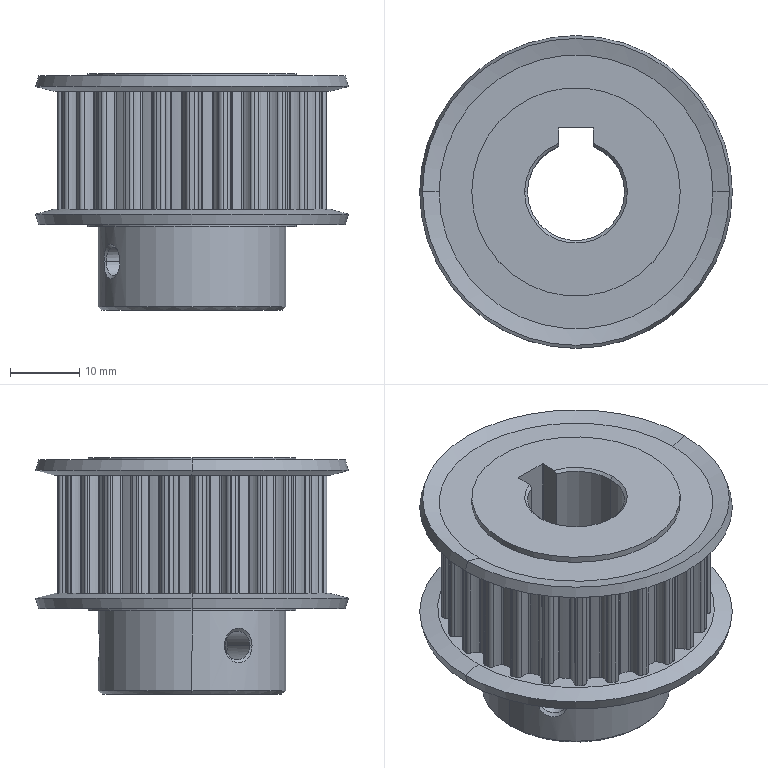Part | SolidWorks | 1 solid | 270 faces | box 45 x 45 x 34 mm | volume 25485 mm3 | cylinder 236 | cone 24 | plane 10 | commonest cylinder face diameters 1.1 x61 0.5 x57 6.55 x53 35.29 x25 38.83 x25 4.134 x4